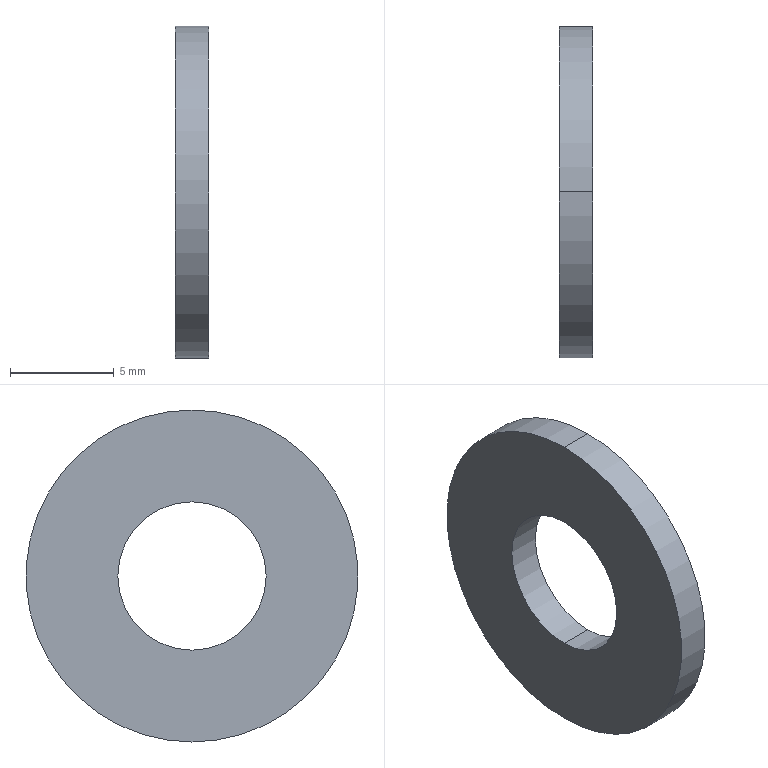Part | SolidWorks | features Extrusion 1 | 1 solid | 6 faces | box 1.6 x 16 x 16 mm | volume 257.457 mm3 | cylinder 4 | plane 2 | commonest cylinder face diameters 7.15 x2 16 x2
STEP:
#1=CARTESIAN_POINT('',(1.6,0.,3.575));
#2=VERTEX_POINT('',#1);
#3=CARTESIAN_POINT('',(1.6,0.,-3.575));
#4=VERTEX_POINT('',#3);
#5=CARTESIAN_POINT('',(1.6,0.,0.));
#6=DIRECTION('',(1.,0.,0.));
#7=DIRECTION('',(0.,0.,-1.));
#8=AXIS2_PLACEMENT_3D('',#5,#6,#7);
#9=CIRCLE('',#8,3.575);
#10=EDGE_CURVE('',#2,#4,#9,.T.);
#11=ORIENTED_EDGE('',*,*,#10,.T.);
#12=CARTESIAN_POINT('',(0.,0.,-3.575));
#13=VERTEX_POINT('',#12);
#14=CARTESIAN_POINT('',(1.6,0.,-3.575));
#15=DIRECTION('',(-1.,0.,0.));
#16=VECTOR('',#15,1000.);
#17=LINE('',#14,#16);
#18=EDGE_CURVE('',#4,#13,#17,.T.);
#19=ORIENTED_EDGE('',*,*,#18,.T.);
#20=CARTESIAN_POINT('',(0.,0.,3.575));
#21=VERTEX_POINT('',#20);
#22=CARTESIAN_POINT('',(0.,0.,0.));
#23=DIRECTION('',(1.,0.,0.));
#24=DIRECTION('',(0.,0.,-1.));
#25=AXIS2_PLACEMENT_3D('',#22,#23,#24);
#26=CIRCLE('',#25,3.575);
#27=EDGE_CURVE('',#21,#13,#26,.T.);
#28=ORIENTED_EDGE('',*,*,#27,.F.);
#29=CARTESIAN_POINT('',(1.6,0.,3.575));
#30=DIRECTION('',(-1.,0.,0.));
#31=VECTOR('',#30,1000.);
#32=LINE('',#29,#31);
#33=EDGE_CURVE('',#2,#21,#32,.T.);
#34=ORIENTED_EDGE('',*,*,#33,.F.);
#35=EDGE_LOOP('',(#11,#19,#28,#34));
#36=FACE_OUTER_BOUND('',#35,.T.);
#37=CARTESIAN_POINT('',(1.6,0.,0.));
#38=DIRECTION('',(-1.,0.,0.));
#39=DIRECTION('',(0.,0.,1.));
#40=AXIS2_PLACEMENT_3D('',#37,#38,#39);
#41=CYLINDRICAL_SURFACE('',#40,3.575);
#42=ADVANCED_FACE('',(#36),#41,.F.);
#43=CARTESIAN_POINT('',(1.6,0.,-8.));
#44=VERTEX_POINT('',#43);
#45=CARTESIAN_POINT('',(1.6,0.,8.));
#46=VERTEX_POINT('',#45);
#47=CARTESIAN_POINT('',(1.6,0.,0.));
#48=DIRECTION('',(1.,0.,0.));
#49=DIRECTION('',(0.,0.,-1.));
#50=AXIS2_PLACEMENT_3D('',#47,#48,#49);
#51=CIRCLE('',#50,8.);
#52=EDGE_CURVE('',#44,#46,#51,.T.);
#53=ORIENTED_EDGE('',*,*,#52,.F.);
#54=CARTESIAN_POINT('',(0.,0.,-8.));
#55=VERTEX_POINT('',#54);
#56=CARTESIAN_POINT('',(1.6,0.,-8.));
#57=DIRECTION('',(-1.,0.,0.));
#58=VECTOR('',#57,1000.);
#59=LINE('',#56,#58);
#60=EDGE_CURVE('',#44,#55,#59,.T.);
#61=ORIENTED_EDGE('',*,*,#60,.T.);
#62=CARTESIAN_POINT('',(0.,0.,8.));
#63=VERTEX_POINT('',#62);
#64=CARTESIAN_POINT('',(0.,0.,0.));
#65=DIRECTION('',(1.,0.,0.));
#66=DIRECTION('',(0.,0.,-1.));
#67=AXIS2_PLACEMENT_3D('',#64,#65,#66);
#68=CIRCLE('',#67,8.);
#69=EDGE_CURVE('',#55,#63,#68,.T.);
#70=ORIENTED_EDGE('',*,*,#69,.T.);
#71=CARTESIAN_POINT('',(1.6,0.,8.));
#72=DIRECTION('',(-1.,0.,0.));
#73=VECTOR('',#72,1000.);
#74=LINE('',#71,#73);
#75=EDGE_CURVE('',#46,#63,#74,.T.);
#76=ORIENTED_EDGE('',*,*,#75,.F.);
#77=EDGE_LOOP('',(#53,#61,#70,#76));
#78=FACE_OUTER_BOUND('',#77,.T.);
#79=CARTESIAN_POINT('',(1.6,0.,0.));
#80=DIRECTION('',(-1.,0.,0.));
#81=DIRECTION('',(0.,0.,1.));
#82=AXIS2_PLACEMENT_3D('',#79,#80,#81);
#83=CYLINDRICAL_SURFACE('',#82,8.);
#84=ADVANCED_FACE('',(#78),#83,.T.);
#85=CARTESIAN_POINT('',(1.6,0.,0.));
#86=DIRECTION('',(1.,0.,0.));
#87=DIRECTION('',(0.,0.,-1.));
#88=AXIS2_PLACEMENT_3D('',#85,#86,#87);
#89=CIRCLE('',#88,8.);
#90=EDGE_CURVE('',#46,#44,#89,.T.);
#91=ORIENTED_EDGE('',*,*,#90,.T.);
#92=ORIENTED_EDGE('',*,*,#52,.T.);
#93=EDGE_LOOP('',(#91,#92));
#94=FACE_OUTER_BOUND('',#93,.T.);
#95=ORIENTED_EDGE('',*,*,#10,.F.);
#96=CARTESIAN_POINT('',(1.6,0.,0.));
#97=DIRECTION('',(1.,0.,0.));
#98=DIRECTION('',(0.,0.,-1.));
#99=AXIS2_PLACEMENT_3D('',#96,#97,#98);
#100=CIRCLE('',#99,3.575);
#101=EDGE_CURVE('',#4,#2,#100,.T.);
#102=ORIENTED_EDGE('',*,*,#101,.F.);
#103=EDGE_LOOP('',(#95,#102));
#104=FACE_BOUND('',#103,.T.);
#105=CARTESIAN_POINT('',(1.6,0.,0.));
#106=DIRECTION('',(1.,0.,0.));
#107=DIRECTION('',(0.,0.,-1.));
#108=AXIS2_PLACEMENT_3D('',#105,#106,#107);
#109=PLANE('',#108);
#110=ADVANCED_FACE('',(#94,#104),#109,.T.);
#111=CARTESIAN_POINT('',(0.,0.,0.));
#112=DIRECTION('',(1.,0.,0.));
#113=DIRECTION('',(0.,0.,-1.));
#114=AXIS2_PLACEMENT_3D('',#111,#112,#113);
#115=CIRCLE('',#114,8.);
#116=EDGE_CURVE('',#63,#55,#115,.T.);
#117=ORIENTED_EDGE('',*,*,#116,.F.);
#118=ORIENTED_EDGE('',*,*,#69,.F.);
#119=EDGE_LOOP('',(#117,#118));
#120=FACE_OUTER_BOUND('',#119,.T.);
#121=ORIENTED_EDGE('',*,*,#27,.T.);
#122=CARTESIAN_POINT('',(0.,0.,0.));
#123=DIRECTION('',(1.,0.,0.));
#124=DIRECTION('',(0.,0.,-1.));
#125=AXIS2_PLACEMENT_3D('',#122,#123,#124);
#126=CIRCLE('',#125,3.575);
#127=EDGE_CURVE('',#13,#21,#126,.T.);
#128=ORIENTED_EDGE('',*,*,#127,.T.);
#129=EDGE_LOOP('',(#121,#128));
#130=FACE_BOUND('',#129,.T.);
#131=CARTESIAN_POINT('',(0.,0.,0.));
#132=DIRECTION('',(1.,0.,0.));
#133=DIRECTION('',(0.,0.,-1.));
#134=AXIS2_PLACEMENT_3D('',#131,#132,#133);
#135=PLANE('',#134);
#136=ADVANCED_FACE('',(#120,#130),#135,.F.);
#137=ORIENTED_EDGE('',*,*,#60,.F.);
#138=ORIENTED_EDGE('',*,*,#90,.F.);
#139=ORIENTED_EDGE('',*,*,#75,.T.);
#140=ORIENTED_EDGE('',*,*,#116,.T.);
#141=EDGE_LOOP('',(#137,#138,#139,#140));
#142=FACE_OUTER_BOUND('',#141,.T.);
#143=CARTESIAN_POINT('',(1.6,0.,0.));
#144=DIRECTION('',(-1.,0.,0.));
#145=DIRECTION('',(0.,0.,1.));
#146=AXIS2_PLACEMENT_3D('',#143,#144,#145);
#147=CYLINDRICAL_SURFACE('',#146,8.);
#148=ADVANCED_FACE('',(#142),#147,.T.);
#149=ORIENTED_EDGE('',*,*,#18,.F.);
#150=ORIENTED_EDGE('',*,*,#101,.T.);
#151=ORIENTED_EDGE('',*,*,#33,.T.);
#152=ORIENTED_EDGE('',*,*,#127,.F.);
#153=EDGE_LOOP('',(#149,#150,#151,#152));
#154=FACE_OUTER_BOUND('',#153,.T.);
#155=CARTESIAN_POINT('',(1.6,0.,0.));
#156=DIRECTION('',(-1.,0.,0.));
#157=DIRECTION('',(0.,0.,1.));
#158=AXIS2_PLACEMENT_3D('',#155,#156,#157);
#159=CYLINDRICAL_SURFACE('',#158,3.575);
#160=ADVANCED_FACE('',(#154),#159,.F.);
#161=CLOSED_SHELL('',(#42,#84,#110,#136,#148,#160));
#162=MANIFOLD_SOLID_BREP('',#161);
#163=CARTESIAN_POINT('',(0.,0.,0.));
#164=DIRECTION('',(0.,0.,1.));
#165=DIRECTION('',(1.,0.,0.));
#166=AXIS2_PLACEMENT_3D('',#163,#164,#165);
#167=(LENGTH_UNIT()NAMED_UNIT(*)SI_UNIT(.MILLI.,.METRE.));
#168=UNCERTAINTY_MEASURE_WITH_UNIT(LENGTH_MEASURE(0.00001),#167,'','');
#169=(NAMED_UNIT(*)PLANE_ANGLE_UNIT()SI_UNIT($,.RADIAN.));
#170=(NAMED_UNIT(*)SI_UNIT($,.STERADIAN.)SOLID_ANGLE_UNIT());
#171=(GEOMETRIC_REPRESENTATION_CONTEXT(3)GLOBAL_UNCERTAINTY_ASSIGNED_CONTEXT((#168))GLOBAL_UNIT_ASSIGNED_CONTEXT((#167,#169,#170))REPRESENTATION_CONTEXT('',''));
#172=ADVANCED_BREP_SHAPE_REPRESENTATION('',(#162,#166),#171);